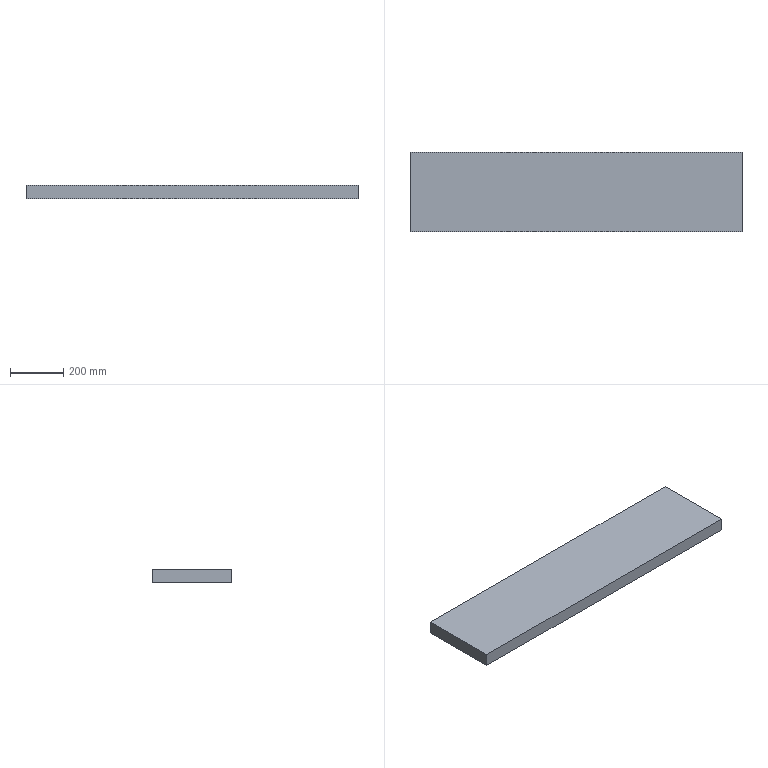Part | SolidWorks | features Extrusion 1 | 1 solid | 6 faces | box 1250 x 300 x 50 mm | volume 18750000 mm3 | plane 6
STEP:
#1=CARTESIAN_POINT('',(-625.,150.,0.));
#2=VERTEX_POINT('',#1);
#3=CARTESIAN_POINT('',(-625.,-150.,0.));
#4=VERTEX_POINT('',#3);
#5=CARTESIAN_POINT('',(-625.,-150.,0.));
#6=DIRECTION('',(0.,-1.,0.));
#7=VECTOR('',#6,1000.);
#8=LINE('',#5,#7);
#9=EDGE_CURVE('',#2,#4,#8,.T.);
#10=ORIENTED_EDGE('',*,*,#9,.T.);
#11=CARTESIAN_POINT('',(-625.,-150.,50.));
#12=VERTEX_POINT('',#11);
#13=CARTESIAN_POINT('',(-625.,-150.,50.));
#14=DIRECTION('',(0.,0.,-1.));
#15=VECTOR('',#14,1000.);
#16=LINE('',#13,#15);
#17=EDGE_CURVE('',#12,#4,#16,.T.);
#18=ORIENTED_EDGE('',*,*,#17,.F.);
#19=CARTESIAN_POINT('',(-625.,150.,50.));
#20=VERTEX_POINT('',#19);
#21=CARTESIAN_POINT('',(-625.,-150.,50.));
#22=DIRECTION('',(0.,-1.,0.));
#23=VECTOR('',#22,1000.);
#24=LINE('',#21,#23);
#25=EDGE_CURVE('',#20,#12,#24,.T.);
#26=ORIENTED_EDGE('',*,*,#25,.F.);
#27=CARTESIAN_POINT('',(-625.,150.,50.));
#28=DIRECTION('',(0.,0.,-1.));
#29=VECTOR('',#28,1000.);
#30=LINE('',#27,#29);
#31=EDGE_CURVE('',#20,#2,#30,.T.);
#32=ORIENTED_EDGE('',*,*,#31,.T.);
#33=EDGE_LOOP('',(#10,#18,#26,#32));
#34=FACE_OUTER_BOUND('',#33,.T.);
#35=CARTESIAN_POINT('',(-625.,-150.,50.));
#36=DIRECTION('',(1.,0.,0.));
#37=DIRECTION('',(0.,0.,-1.));
#38=AXIS2_PLACEMENT_3D('',#35,#36,#37);
#39=PLANE('',#38);
#40=ADVANCED_FACE('',(#34),#39,.F.);
#41=CARTESIAN_POINT('',(625.,-150.,0.));
#42=VERTEX_POINT('',#41);
#43=CARTESIAN_POINT('',(625.,-150.,0.));
#44=DIRECTION('',(1.,0.,0.));
#45=VECTOR('',#44,1000.);
#46=LINE('',#43,#45);
#47=EDGE_CURVE('',#4,#42,#46,.T.);
#48=ORIENTED_EDGE('',*,*,#47,.T.);
#49=CARTESIAN_POINT('',(625.,-150.,50.));
#50=VERTEX_POINT('',#49);
#51=CARTESIAN_POINT('',(625.,-150.,50.));
#52=DIRECTION('',(0.,0.,-1.));
#53=VECTOR('',#52,1000.);
#54=LINE('',#51,#53);
#55=EDGE_CURVE('',#50,#42,#54,.T.);
#56=ORIENTED_EDGE('',*,*,#55,.F.);
#57=CARTESIAN_POINT('',(625.,-150.,50.));
#58=DIRECTION('',(1.,0.,0.));
#59=VECTOR('',#58,1000.);
#60=LINE('',#57,#59);
#61=EDGE_CURVE('',#12,#50,#60,.T.);
#62=ORIENTED_EDGE('',*,*,#61,.F.);
#63=ORIENTED_EDGE('',*,*,#17,.T.);
#64=EDGE_LOOP('',(#48,#56,#62,#63));
#65=FACE_OUTER_BOUND('',#64,.T.);
#66=CARTESIAN_POINT('',(625.,-150.,50.));
#67=DIRECTION('',(0.,1.,0.));
#68=DIRECTION('',(-1.,0.,0.));
#69=AXIS2_PLACEMENT_3D('',#66,#67,#68);
#70=PLANE('',#69);
#71=ADVANCED_FACE('',(#65),#70,.F.);
#72=CARTESIAN_POINT('',(625.,150.,0.));
#73=VERTEX_POINT('',#72);
#74=CARTESIAN_POINT('',(625.,-150.,0.));
#75=DIRECTION('',(0.,1.,0.));
#76=VECTOR('',#75,1000.);
#77=LINE('',#74,#76);
#78=EDGE_CURVE('',#42,#73,#77,.T.);
#79=ORIENTED_EDGE('',*,*,#78,.T.);
#80=CARTESIAN_POINT('',(625.,150.,50.));
#81=VERTEX_POINT('',#80);
#82=CARTESIAN_POINT('',(625.,150.,50.));
#83=DIRECTION('',(0.,0.,-1.));
#84=VECTOR('',#83,1000.);
#85=LINE('',#82,#84);
#86=EDGE_CURVE('',#81,#73,#85,.T.);
#87=ORIENTED_EDGE('',*,*,#86,.F.);
#88=CARTESIAN_POINT('',(625.,-150.,50.));
#89=DIRECTION('',(0.,1.,0.));
#90=VECTOR('',#89,1000.);
#91=LINE('',#88,#90);
#92=EDGE_CURVE('',#50,#81,#91,.T.);
#93=ORIENTED_EDGE('',*,*,#92,.F.);
#94=ORIENTED_EDGE('',*,*,#55,.T.);
#95=EDGE_LOOP('',(#79,#87,#93,#94));
#96=FACE_OUTER_BOUND('',#95,.T.);
#97=CARTESIAN_POINT('',(625.,-150.,50.));
#98=DIRECTION('',(-1.,0.,0.));
#99=DIRECTION('',(0.,0.,1.));
#100=AXIS2_PLACEMENT_3D('',#97,#98,#99);
#101=PLANE('',#100);
#102=ADVANCED_FACE('',(#96),#101,.F.);
#103=CARTESIAN_POINT('',(625.,150.,0.));
#104=DIRECTION('',(-1.,0.,0.));
#105=VECTOR('',#104,1000.);
#106=LINE('',#103,#105);
#107=EDGE_CURVE('',#73,#2,#106,.T.);
#108=ORIENTED_EDGE('',*,*,#107,.T.);
#109=ORIENTED_EDGE('',*,*,#31,.F.);
#110=CARTESIAN_POINT('',(625.,150.,50.));
#111=DIRECTION('',(-1.,0.,0.));
#112=VECTOR('',#111,1000.);
#113=LINE('',#110,#112);
#114=EDGE_CURVE('',#81,#20,#113,.T.);
#115=ORIENTED_EDGE('',*,*,#114,.F.);
#116=ORIENTED_EDGE('',*,*,#86,.T.);
#117=EDGE_LOOP('',(#108,#109,#115,#116));
#118=FACE_OUTER_BOUND('',#117,.T.);
#119=CARTESIAN_POINT('',(625.,150.,50.));
#120=DIRECTION('',(0.,-1.,0.));
#121=DIRECTION('',(1.,0.,0.));
#122=AXIS2_PLACEMENT_3D('',#119,#120,#121);
#123=PLANE('',#122);
#124=ADVANCED_FACE('',(#118),#123,.F.);
#125=ORIENTED_EDGE('',*,*,#25,.T.);
#126=ORIENTED_EDGE('',*,*,#61,.T.);
#127=ORIENTED_EDGE('',*,*,#92,.T.);
#128=ORIENTED_EDGE('',*,*,#114,.T.);
#129=EDGE_LOOP('',(#125,#126,#127,#128));
#130=FACE_OUTER_BOUND('',#129,.T.);
#131=CARTESIAN_POINT('',(0.,0.,50.));
#132=DIRECTION('',(0.,0.,1.));
#133=DIRECTION('',(1.,0.,0.));
#134=AXIS2_PLACEMENT_3D('',#131,#132,#133);
#135=PLANE('',#134);
#136=ADVANCED_FACE('',(#130),#135,.T.);
#137=ORIENTED_EDGE('',*,*,#9,.F.);
#138=ORIENTED_EDGE('',*,*,#107,.F.);
#139=ORIENTED_EDGE('',*,*,#78,.F.);
#140=ORIENTED_EDGE('',*,*,#47,.F.);
#141=EDGE_LOOP('',(#137,#138,#139,#140));
#142=FACE_OUTER_BOUND('',#141,.T.);
#143=CARTESIAN_POINT('',(0.,0.,0.));
#144=DIRECTION('',(0.,0.,1.));
#145=DIRECTION('',(1.,0.,0.));
#146=AXIS2_PLACEMENT_3D('',#143,#144,#145);
#147=PLANE('',#146);
#148=ADVANCED_FACE('',(#142),#147,.F.);
#149=CLOSED_SHELL('',(#40,#71,#102,#124,#136,#148));
#150=MANIFOLD_SOLID_BREP('',#149);
#151=CARTESIAN_POINT('',(0.,0.,0.));
#152=DIRECTION('',(0.,0.,1.));
#153=DIRECTION('',(1.,0.,0.));
#154=AXIS2_PLACEMENT_3D('',#151,#152,#153);
#155=(LENGTH_UNIT()NAMED_UNIT(*)SI_UNIT(.MILLI.,.METRE.));
#156=UNCERTAINTY_MEASURE_WITH_UNIT(LENGTH_MEASURE(0.00001),#155,'','');
#157=(NAMED_UNIT(*)PLANE_ANGLE_UNIT()SI_UNIT($,.RADIAN.));
#158=(NAMED_UNIT(*)SI_UNIT($,.STERADIAN.)SOLID_ANGLE_UNIT());
#159=(GEOMETRIC_REPRESENTATION_CONTEXT(3)GLOBAL_UNCERTAINTY_ASSIGNED_CONTEXT((#156))GLOBAL_UNIT_ASSIGNED_CONTEXT((#155,#157,#158))REPRESENTATION_CONTEXT('',''));
#160=ADVANCED_BREP_SHAPE_REPRESENTATION('',(#150,#154),#159);